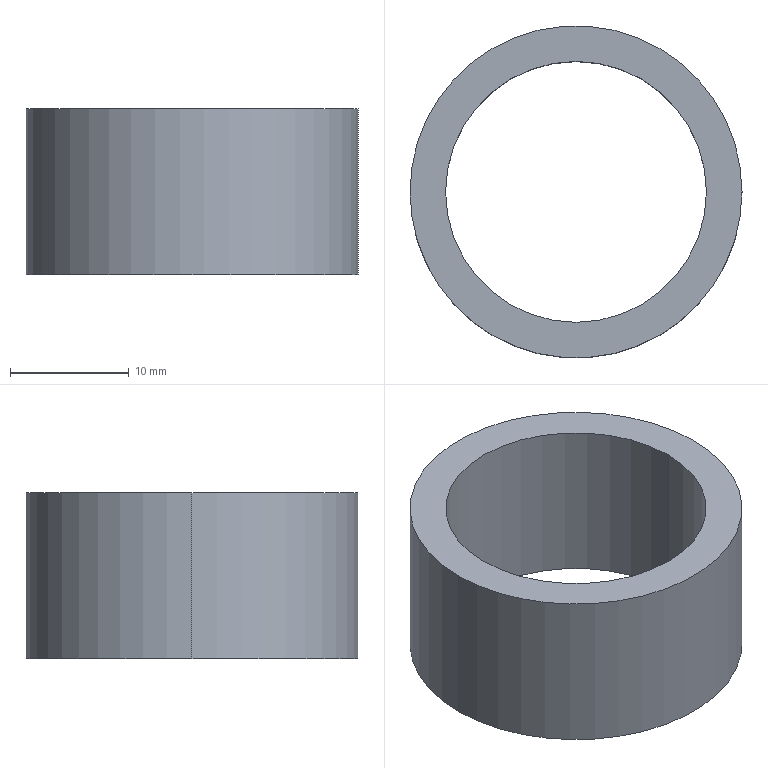Part | STEP file | Shaft collar | 1 solid | 6 faces | box 28 x 28 x 14 mm | volume 3299 mm3 | cylinder 4 | plane 2 | commonest cylinder face diameters 22 x2 28 x2
STEP:
#1=CARTESIAN_POINT('',(-11.,0.,14.));
#2=VERTEX_POINT('',#1);
#3=CARTESIAN_POINT('',(11.,0.,14.));
#4=VERTEX_POINT('',#3);
#5=CARTESIAN_POINT('',(0.,0.,14.));
#6=DIRECTION('',(0.,0.,1.));
#7=DIRECTION('',(1.,0.,0.));
#8=AXIS2_PLACEMENT_3D('',#5,#6,#7);
#9=CIRCLE('',#8,11.);
#10=EDGE_CURVE('',#2,#4,#9,.T.);
#11=ORIENTED_EDGE('',*,*,#10,.T.);
#12=CARTESIAN_POINT('',(11.,0.,0.));
#13=VERTEX_POINT('',#12);
#14=CARTESIAN_POINT('',(11.,0.,14.));
#15=DIRECTION('',(0.,0.,-1.));
#16=VECTOR('',#15,1000.);
#17=LINE('',#14,#16);
#18=EDGE_CURVE('',#4,#13,#17,.T.);
#19=ORIENTED_EDGE('',*,*,#18,.T.);
#20=CARTESIAN_POINT('',(-11.,0.,0.));
#21=VERTEX_POINT('',#20);
#22=CARTESIAN_POINT('',(0.,0.,0.));
#23=DIRECTION('',(0.,0.,1.));
#24=DIRECTION('',(1.,0.,0.));
#25=AXIS2_PLACEMENT_3D('',#22,#23,#24);
#26=CIRCLE('',#25,11.);
#27=EDGE_CURVE('',#21,#13,#26,.T.);
#28=ORIENTED_EDGE('',*,*,#27,.F.);
#29=CARTESIAN_POINT('',(-11.,0.,14.));
#30=DIRECTION('',(0.,0.,-1.));
#31=VECTOR('',#30,1000.);
#32=LINE('',#29,#31);
#33=EDGE_CURVE('',#2,#21,#32,.T.);
#34=ORIENTED_EDGE('',*,*,#33,.F.);
#35=EDGE_LOOP('',(#11,#19,#28,#34));
#36=FACE_OUTER_BOUND('',#35,.T.);
#37=CARTESIAN_POINT('',(0.,0.,14.));
#38=DIRECTION('',(0.,0.,-1.));
#39=DIRECTION('',(-1.,0.,0.));
#40=AXIS2_PLACEMENT_3D('',#37,#38,#39);
#41=CYLINDRICAL_SURFACE('',#40,11.);
#42=ADVANCED_FACE('',(#36),#41,.F.);
#43=CARTESIAN_POINT('',(14.,0.,14.));
#44=VERTEX_POINT('',#43);
#45=CARTESIAN_POINT('',(-14.,0.,14.));
#46=VERTEX_POINT('',#45);
#47=CARTESIAN_POINT('',(0.,0.,14.));
#48=DIRECTION('',(0.,0.,1.));
#49=DIRECTION('',(1.,0.,0.));
#50=AXIS2_PLACEMENT_3D('',#47,#48,#49);
#51=CIRCLE('',#50,14.);
#52=EDGE_CURVE('',#44,#46,#51,.T.);
#53=ORIENTED_EDGE('',*,*,#52,.F.);
#54=CARTESIAN_POINT('',(14.,0.,0.));
#55=VERTEX_POINT('',#54);
#56=CARTESIAN_POINT('',(14.,0.,14.));
#57=DIRECTION('',(0.,0.,-1.));
#58=VECTOR('',#57,1000.);
#59=LINE('',#56,#58);
#60=EDGE_CURVE('',#44,#55,#59,.T.);
#61=ORIENTED_EDGE('',*,*,#60,.T.);
#62=CARTESIAN_POINT('',(-14.,0.,0.));
#63=VERTEX_POINT('',#62);
#64=CARTESIAN_POINT('',(0.,0.,0.));
#65=DIRECTION('',(0.,0.,1.));
#66=DIRECTION('',(1.,0.,0.));
#67=AXIS2_PLACEMENT_3D('',#64,#65,#66);
#68=CIRCLE('',#67,14.);
#69=EDGE_CURVE('',#55,#63,#68,.T.);
#70=ORIENTED_EDGE('',*,*,#69,.T.);
#71=CARTESIAN_POINT('',(-14.,0.,14.));
#72=DIRECTION('',(0.,0.,-1.));
#73=VECTOR('',#72,1000.);
#74=LINE('',#71,#73);
#75=EDGE_CURVE('',#46,#63,#74,.T.);
#76=ORIENTED_EDGE('',*,*,#75,.F.);
#77=EDGE_LOOP('',(#53,#61,#70,#76));
#78=FACE_OUTER_BOUND('',#77,.T.);
#79=CARTESIAN_POINT('',(0.,0.,14.));
#80=DIRECTION('',(0.,0.,-1.));
#81=DIRECTION('',(-1.,0.,0.));
#82=AXIS2_PLACEMENT_3D('',#79,#80,#81);
#83=CYLINDRICAL_SURFACE('',#82,14.);
#84=ADVANCED_FACE('',(#78),#83,.T.);
#85=CARTESIAN_POINT('',(0.,0.,14.));
#86=DIRECTION('',(0.,0.,1.));
#87=DIRECTION('',(1.,0.,0.));
#88=AXIS2_PLACEMENT_3D('',#85,#86,#87);
#89=CIRCLE('',#88,14.);
#90=EDGE_CURVE('',#46,#44,#89,.T.);
#91=ORIENTED_EDGE('',*,*,#90,.T.);
#92=ORIENTED_EDGE('',*,*,#52,.T.);
#93=EDGE_LOOP('',(#91,#92));
#94=FACE_OUTER_BOUND('',#93,.T.);
#95=ORIENTED_EDGE('',*,*,#10,.F.);
#96=CARTESIAN_POINT('',(0.,0.,14.));
#97=DIRECTION('',(0.,0.,1.));
#98=DIRECTION('',(1.,0.,0.));
#99=AXIS2_PLACEMENT_3D('',#96,#97,#98);
#100=CIRCLE('',#99,11.);
#101=EDGE_CURVE('',#4,#2,#100,.T.);
#102=ORIENTED_EDGE('',*,*,#101,.F.);
#103=EDGE_LOOP('',(#95,#102));
#104=FACE_BOUND('',#103,.T.);
#105=CARTESIAN_POINT('',(0.,0.,14.));
#106=DIRECTION('',(0.,0.,1.));
#107=DIRECTION('',(1.,0.,0.));
#108=AXIS2_PLACEMENT_3D('',#105,#106,#107);
#109=PLANE('',#108);
#110=ADVANCED_FACE('',(#94,#104),#109,.T.);
#111=CARTESIAN_POINT('',(0.,0.,0.));
#112=DIRECTION('',(0.,0.,1.));
#113=DIRECTION('',(1.,0.,0.));
#114=AXIS2_PLACEMENT_3D('',#111,#112,#113);
#115=CIRCLE('',#114,14.);
#116=EDGE_CURVE('',#63,#55,#115,.T.);
#117=ORIENTED_EDGE('',*,*,#116,.F.);
#118=ORIENTED_EDGE('',*,*,#69,.F.);
#119=EDGE_LOOP('',(#117,#118));
#120=FACE_OUTER_BOUND('',#119,.T.);
#121=ORIENTED_EDGE('',*,*,#27,.T.);
#122=CARTESIAN_POINT('',(0.,0.,0.));
#123=DIRECTION('',(0.,0.,1.));
#124=DIRECTION('',(1.,0.,0.));
#125=AXIS2_PLACEMENT_3D('',#122,#123,#124);
#126=CIRCLE('',#125,11.);
#127=EDGE_CURVE('',#13,#21,#126,.T.);
#128=ORIENTED_EDGE('',*,*,#127,.T.);
#129=EDGE_LOOP('',(#121,#128));
#130=FACE_BOUND('',#129,.T.);
#131=CARTESIAN_POINT('',(0.,0.,0.));
#132=DIRECTION('',(0.,0.,1.));
#133=DIRECTION('',(1.,0.,0.));
#134=AXIS2_PLACEMENT_3D('',#131,#132,#133);
#135=PLANE('',#134);
#136=ADVANCED_FACE('',(#120,#130),#135,.F.);
#137=ORIENTED_EDGE('',*,*,#60,.F.);
#138=ORIENTED_EDGE('',*,*,#90,.F.);
#139=ORIENTED_EDGE('',*,*,#75,.T.);
#140=ORIENTED_EDGE('',*,*,#116,.T.);
#141=EDGE_LOOP('',(#137,#138,#139,#140));
#142=FACE_OUTER_BOUND('',#141,.T.);
#143=CARTESIAN_POINT('',(0.,0.,14.));
#144=DIRECTION('',(0.,0.,-1.));
#145=DIRECTION('',(-1.,0.,0.));
#146=AXIS2_PLACEMENT_3D('',#143,#144,#145);
#147=CYLINDRICAL_SURFACE('',#146,14.);
#148=ADVANCED_FACE('',(#142),#147,.T.);
#149=ORIENTED_EDGE('',*,*,#18,.F.);
#150=ORIENTED_EDGE('',*,*,#101,.T.);
#151=ORIENTED_EDGE('',*,*,#33,.T.);
#152=ORIENTED_EDGE('',*,*,#127,.F.);
#153=EDGE_LOOP('',(#149,#150,#151,#152));
#154=FACE_OUTER_BOUND('',#153,.T.);
#155=CARTESIAN_POINT('',(0.,0.,14.));
#156=DIRECTION('',(0.,0.,-1.));
#157=DIRECTION('',(-1.,0.,0.));
#158=AXIS2_PLACEMENT_3D('',#155,#156,#157);
#159=CYLINDRICAL_SURFACE('',#158,11.);
#160=ADVANCED_FACE('',(#154),#159,.F.);
#161=CLOSED_SHELL('',(#42,#84,#110,#136,#148,#160));
#162=MANIFOLD_SOLID_BREP('',#161);
#163=CARTESIAN_POINT('',(0.,0.,0.));
#164=DIRECTION('',(0.,0.,1.));
#165=DIRECTION('',(1.,0.,0.));
#166=AXIS2_PLACEMENT_3D('',#163,#164,#165);
#167=(LENGTH_UNIT()NAMED_UNIT(*)SI_UNIT(.MILLI.,.METRE.));
#168=UNCERTAINTY_MEASURE_WITH_UNIT(LENGTH_MEASURE(0.00001),#167,'','');
#169=(NAMED_UNIT(*)PLANE_ANGLE_UNIT()SI_UNIT($,.RADIAN.));
#170=(NAMED_UNIT(*)SI_UNIT($,.STERADIAN.)SOLID_ANGLE_UNIT());
#171=(GEOMETRIC_REPRESENTATION_CONTEXT(3)GLOBAL_UNCERTAINTY_ASSIGNED_CONTEXT((#168))GLOBAL_UNIT_ASSIGNED_CONTEXT((#167,#169,#170))REPRESENTATION_CONTEXT('',''));
#172=ADVANCED_BREP_SHAPE_REPRESENTATION('',(#162,#166),#171);